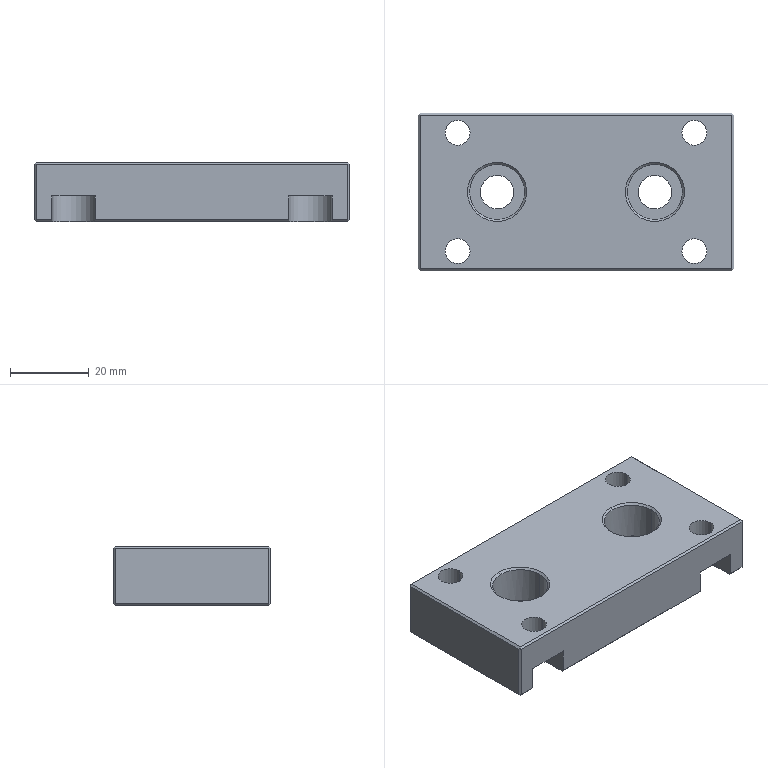Part | STEP file | Roll shaft support base plate | 1 solid | 76 faces | box 80 x 40 x 15 mm | volume 40545 mm3 | plane 44 | cylinder 20 | cone 12 | commonest cylinder face diameters 6.3 x8 8.5 x4 11 x4 14 x4